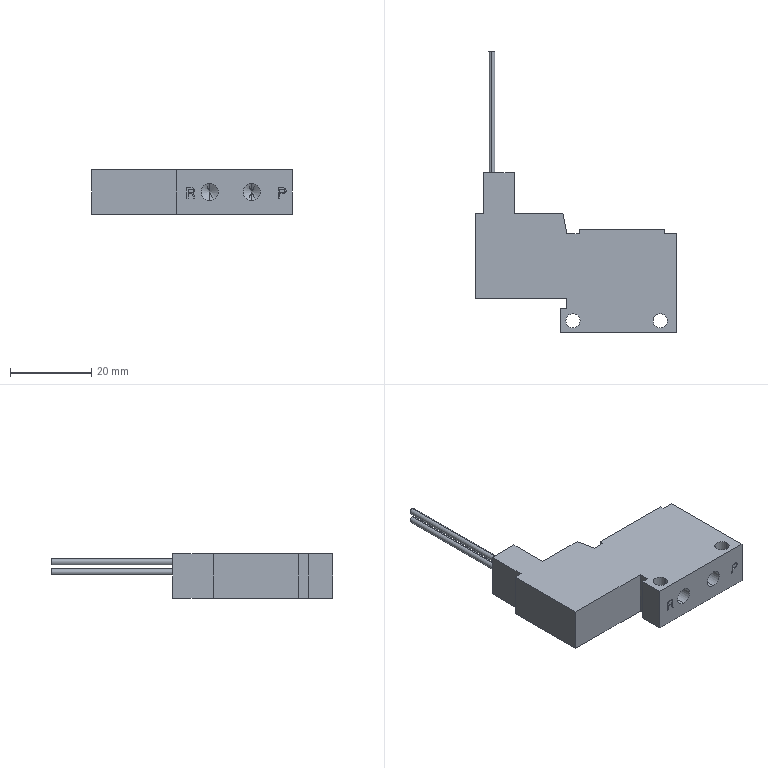Part | STEP file | 1 solid | 100 faces | box 49.5 x 69.5 x 11 mm | volume 13145 mm3 | plane 76 | cylinder 16 | cone 8 | commonest cylinder face diameters 4.2 x8 1.5 x4 3.5 x4